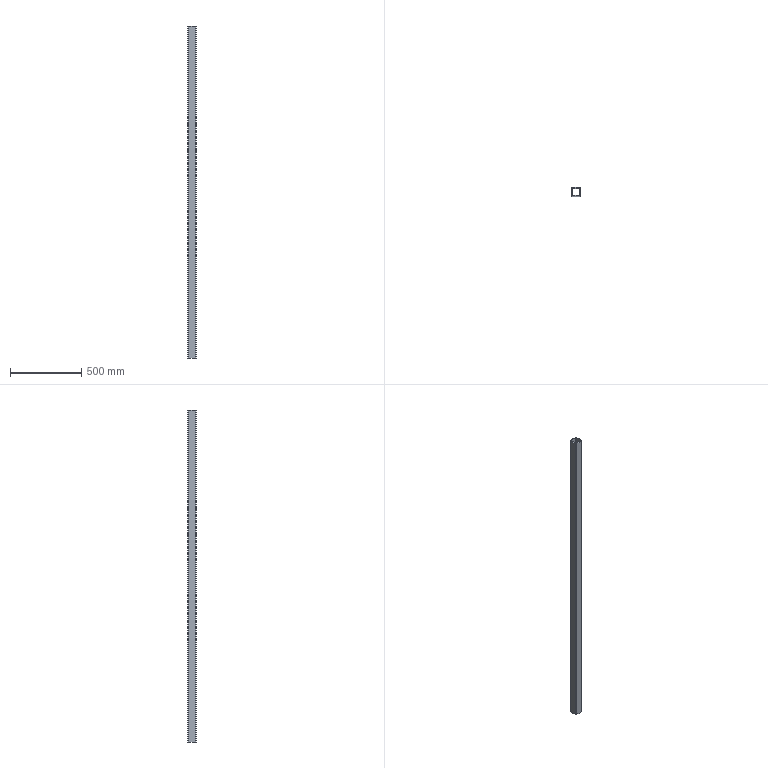Part | SolidWorks | features Fillet 2, Extrusion 1 | 1 solid | 18 faces | box 60 x 60 x 2330 mm | volume 2033678 mm3 | plane 10 | cylinder 8 | commonest cylinder face diameters 6 x4 12 x4
STEP:
#1=CARTESIAN_POINT('',(-24.,-30.,1165.));
#2=VERTEX_POINT('',#1);
#3=CARTESIAN_POINT('',(24.,-30.,1165.));
#4=VERTEX_POINT('',#3);
#5=CARTESIAN_POINT('',(-30.,-30.,1165.));
#6=DIRECTION('',(1.,0.,0.));
#7=VECTOR('',#6,1000.);
#8=LINE('',#5,#7);
#9=EDGE_CURVE('',#2,#4,#8,.T.);
#10=ORIENTED_EDGE('',*,*,#9,.T.);
#11=CARTESIAN_POINT('',(30.,-24.,1165.));
#12=VERTEX_POINT('',#11);
#13=CARTESIAN_POINT('',(24.,-24.,1165.));
#14=DIRECTION('',(0.,0.,1.));
#15=DIRECTION('',(-1.,0.,0.));
#16=AXIS2_PLACEMENT_3D('',#13,#14,#15);
#17=CIRCLE('',#16,6.);
#18=EDGE_CURVE('',#4,#12,#17,.T.);
#19=ORIENTED_EDGE('',*,*,#18,.T.);
#20=CARTESIAN_POINT('',(30.,24.,1165.));
#21=VERTEX_POINT('',#20);
#22=CARTESIAN_POINT('',(30.,-30.,1165.));
#23=DIRECTION('',(0.,1.,0.));
#24=VECTOR('',#23,1000.);
#25=LINE('',#22,#24);
#26=EDGE_CURVE('',#12,#21,#25,.T.);
#27=ORIENTED_EDGE('',*,*,#26,.T.);
#28=CARTESIAN_POINT('',(24.,30.,1165.));
#29=VERTEX_POINT('',#28);
#30=CARTESIAN_POINT('',(24.,24.,1165.));
#31=DIRECTION('',(0.,0.,1.));
#32=DIRECTION('',(-1.,0.,0.));
#33=AXIS2_PLACEMENT_3D('',#30,#31,#32);
#34=CIRCLE('',#33,6.);
#35=EDGE_CURVE('',#21,#29,#34,.T.);
#36=ORIENTED_EDGE('',*,*,#35,.T.);
#37=CARTESIAN_POINT('',(-24.,30.,1165.));
#38=VERTEX_POINT('',#37);
#39=CARTESIAN_POINT('',(-30.,30.,1165.));
#40=DIRECTION('',(-1.,0.,0.));
#41=VECTOR('',#40,1000.);
#42=LINE('',#39,#41);
#43=EDGE_CURVE('',#29,#38,#42,.T.);
#44=ORIENTED_EDGE('',*,*,#43,.T.);
#45=CARTESIAN_POINT('',(-30.,24.,1165.));
#46=VERTEX_POINT('',#45);
#47=CARTESIAN_POINT('',(-24.,24.,1165.));
#48=DIRECTION('',(0.,0.,1.));
#49=DIRECTION('',(-1.,0.,0.));
#50=AXIS2_PLACEMENT_3D('',#47,#48,#49);
#51=CIRCLE('',#50,6.);
#52=EDGE_CURVE('',#38,#46,#51,.T.);
#53=ORIENTED_EDGE('',*,*,#52,.T.);
#54=CARTESIAN_POINT('',(-30.,-24.,1165.));
#55=VERTEX_POINT('',#54);
#56=CARTESIAN_POINT('',(-30.,-30.,1165.));
#57=DIRECTION('',(0.,-1.,0.));
#58=VECTOR('',#57,1000.);
#59=LINE('',#56,#58);
#60=EDGE_CURVE('',#46,#55,#59,.T.);
#61=ORIENTED_EDGE('',*,*,#60,.T.);
#62=CARTESIAN_POINT('',(-24.,-24.,1165.));
#63=DIRECTION('',(0.,0.,1.));
#64=DIRECTION('',(-1.,0.,0.));
#65=AXIS2_PLACEMENT_3D('',#62,#63,#64);
#66=CIRCLE('',#65,6.);
#67=EDGE_CURVE('',#55,#2,#66,.T.);
#68=ORIENTED_EDGE('',*,*,#67,.T.);
#69=EDGE_LOOP('',(#10,#19,#27,#36,#44,#53,#61,#68));
#70=FACE_OUTER_BOUND('',#69,.T.);
#71=CARTESIAN_POINT('',(26.,-23.,1165.));
#72=VERTEX_POINT('',#71);
#73=CARTESIAN_POINT('',(26.,23.,1165.));
#74=VERTEX_POINT('',#73);
#75=CARTESIAN_POINT('',(26.,-26.,1165.));
#76=DIRECTION('',(0.,1.,0.));
#77=VECTOR('',#76,1000.);
#78=LINE('',#75,#77);
#79=EDGE_CURVE('',#72,#74,#78,.T.);
#80=ORIENTED_EDGE('',*,*,#79,.F.);
#81=CARTESIAN_POINT('',(23.,-26.,1165.));
#82=VERTEX_POINT('',#81);
#83=CARTESIAN_POINT('',(23.,-23.,1165.));
#84=DIRECTION('',(0.,0.,-1.));
#85=DIRECTION('',(-1.,0.,0.));
#86=AXIS2_PLACEMENT_3D('',#83,#84,#85);
#87=CIRCLE('',#86,3.);
#88=EDGE_CURVE('',#72,#82,#87,.T.);
#89=ORIENTED_EDGE('',*,*,#88,.T.);
#90=CARTESIAN_POINT('',(-23.,-26.,1165.));
#91=VERTEX_POINT('',#90);
#92=CARTESIAN_POINT('',(-26.,-26.,1165.));
#93=DIRECTION('',(1.,0.,0.));
#94=VECTOR('',#93,1000.);
#95=LINE('',#92,#94);
#96=EDGE_CURVE('',#91,#82,#95,.T.);
#97=ORIENTED_EDGE('',*,*,#96,.F.);
#98=CARTESIAN_POINT('',(-26.,-23.,1165.));
#99=VERTEX_POINT('',#98);
#100=CARTESIAN_POINT('',(-23.,-23.,1165.));
#101=DIRECTION('',(0.,0.,-1.));
#102=DIRECTION('',(-1.,0.,0.));
#103=AXIS2_PLACEMENT_3D('',#100,#101,#102);
#104=CIRCLE('',#103,3.);
#105=EDGE_CURVE('',#91,#99,#104,.T.);
#106=ORIENTED_EDGE('',*,*,#105,.T.);
#107=CARTESIAN_POINT('',(-26.,23.,1165.));
#108=VERTEX_POINT('',#107);
#109=CARTESIAN_POINT('',(-26.,-26.,1165.));
#110=DIRECTION('',(0.,-1.,0.));
#111=VECTOR('',#110,1000.);
#112=LINE('',#109,#111);
#113=EDGE_CURVE('',#108,#99,#112,.T.);
#114=ORIENTED_EDGE('',*,*,#113,.F.);
#115=CARTESIAN_POINT('',(-23.,26.,1165.));
#116=VERTEX_POINT('',#115);
#117=CARTESIAN_POINT('',(-23.,23.,1165.));
#118=DIRECTION('',(0.,0.,-1.));
#119=DIRECTION('',(-1.,0.,0.));
#120=AXIS2_PLACEMENT_3D('',#117,#118,#119);
#121=CIRCLE('',#120,3.);
#122=EDGE_CURVE('',#108,#116,#121,.T.);
#123=ORIENTED_EDGE('',*,*,#122,.T.);
#124=CARTESIAN_POINT('',(23.,26.,1165.));
#125=VERTEX_POINT('',#124);
#126=CARTESIAN_POINT('',(-26.,26.,1165.));
#127=DIRECTION('',(-1.,0.,0.));
#128=VECTOR('',#127,1000.);
#129=LINE('',#126,#128);
#130=EDGE_CURVE('',#125,#116,#129,.T.);
#131=ORIENTED_EDGE('',*,*,#130,.F.);
#132=CARTESIAN_POINT('',(23.,23.,1165.));
#133=DIRECTION('',(0.,0.,-1.));
#134=DIRECTION('',(-1.,0.,0.));
#135=AXIS2_PLACEMENT_3D('',#132,#133,#134);
#136=CIRCLE('',#135,3.);
#137=EDGE_CURVE('',#125,#74,#136,.T.);
#138=ORIENTED_EDGE('',*,*,#137,.T.);
#139=EDGE_LOOP('',(#80,#89,#97,#106,#114,#123,#131,#138));
#140=FACE_BOUND('',#139,.T.);
#141=CARTESIAN_POINT('',(0.,0.,1165.));
#142=DIRECTION('',(0.,0.,-1.));
#143=DIRECTION('',(-1.,0.,0.));
#144=AXIS2_PLACEMENT_3D('',#141,#142,#143);
#145=PLANE('',#144);
#146=ADVANCED_FACE('',(#70,#140),#145,.F.);
#147=CARTESIAN_POINT('',(30.,-24.,-1165.));
#148=VERTEX_POINT('',#147);
#149=CARTESIAN_POINT('',(30.,24.,-1165.));
#150=VERTEX_POINT('',#149);
#151=CARTESIAN_POINT('',(30.,-30.,-1165.));
#152=DIRECTION('',(0.,1.,0.));
#153=VECTOR('',#152,1000.);
#154=LINE('',#151,#153);
#155=EDGE_CURVE('',#148,#150,#154,.T.);
#156=ORIENTED_EDGE('',*,*,#155,.F.);
#157=CARTESIAN_POINT('',(24.,-30.,-1165.));
#158=VERTEX_POINT('',#157);
#159=CARTESIAN_POINT('',(24.,-24.,-1165.));
#160=DIRECTION('',(0.,0.,-1.));
#161=DIRECTION('',(-1.,0.,0.));
#162=AXIS2_PLACEMENT_3D('',#159,#160,#161);
#163=CIRCLE('',#162,6.);
#164=EDGE_CURVE('',#148,#158,#163,.T.);
#165=ORIENTED_EDGE('',*,*,#164,.T.);
#166=CARTESIAN_POINT('',(-24.,-30.,-1165.));
#167=VERTEX_POINT('',#166);
#168=CARTESIAN_POINT('',(-30.,-30.,-1165.));
#169=DIRECTION('',(1.,0.,0.));
#170=VECTOR('',#169,1000.);
#171=LINE('',#168,#170);
#172=EDGE_CURVE('',#167,#158,#171,.T.);
#173=ORIENTED_EDGE('',*,*,#172,.F.);
#174=CARTESIAN_POINT('',(-30.,-24.,-1165.));
#175=VERTEX_POINT('',#174);
#176=CARTESIAN_POINT('',(-24.,-24.,-1165.));
#177=DIRECTION('',(0.,0.,-1.));
#178=DIRECTION('',(-1.,0.,0.));
#179=AXIS2_PLACEMENT_3D('',#176,#177,#178);
#180=CIRCLE('',#179,6.);
#181=EDGE_CURVE('',#167,#175,#180,.T.);
#182=ORIENTED_EDGE('',*,*,#181,.T.);
#183=CARTESIAN_POINT('',(-30.,24.,-1165.));
#184=VERTEX_POINT('',#183);
#185=CARTESIAN_POINT('',(-30.,-30.,-1165.));
#186=DIRECTION('',(0.,-1.,0.));
#187=VECTOR('',#186,1000.);
#188=LINE('',#185,#187);
#189=EDGE_CURVE('',#184,#175,#188,.T.);
#190=ORIENTED_EDGE('',*,*,#189,.F.);
#191=CARTESIAN_POINT('',(-24.,30.,-1165.));
#192=VERTEX_POINT('',#191);
#193=CARTESIAN_POINT('',(-24.,24.,-1165.));
#194=DIRECTION('',(0.,0.,-1.));
#195=DIRECTION('',(-1.,0.,0.));
#196=AXIS2_PLACEMENT_3D('',#193,#194,#195);
#197=CIRCLE('',#196,6.);
#198=EDGE_CURVE('',#184,#192,#197,.T.);
#199=ORIENTED_EDGE('',*,*,#198,.T.);
#200=CARTESIAN_POINT('',(24.,30.,-1165.));
#201=VERTEX_POINT('',#200);
#202=CARTESIAN_POINT('',(-30.,30.,-1165.));
#203=DIRECTION('',(-1.,0.,0.));
#204=VECTOR('',#203,1000.);
#205=LINE('',#202,#204);
#206=EDGE_CURVE('',#201,#192,#205,.T.);
#207=ORIENTED_EDGE('',*,*,#206,.F.);
#208=CARTESIAN_POINT('',(24.,24.,-1165.));
#209=DIRECTION('',(0.,0.,-1.));
#210=DIRECTION('',(-1.,0.,0.));
#211=AXIS2_PLACEMENT_3D('',#208,#209,#210);
#212=CIRCLE('',#211,6.);
#213=EDGE_CURVE('',#201,#150,#212,.T.);
#214=ORIENTED_EDGE('',*,*,#213,.T.);
#215=EDGE_LOOP('',(#156,#165,#173,#182,#190,#199,#207,#214));
#216=FACE_OUTER_BOUND('',#215,.T.);
#217=CARTESIAN_POINT('',(-26.,23.,-1165.));
#218=VERTEX_POINT('',#217);
#219=CARTESIAN_POINT('',(-26.,-23.,-1165.));
#220=VERTEX_POINT('',#219);
#221=CARTESIAN_POINT('',(-26.,-26.,-1165.));
#222=DIRECTION('',(0.,-1.,0.));
#223=VECTOR('',#222,1000.);
#224=LINE('',#221,#223);
#225=EDGE_CURVE('',#218,#220,#224,.T.);
#226=ORIENTED_EDGE('',*,*,#225,.T.);
#227=CARTESIAN_POINT('',(-23.,-26.,-1165.));
#228=VERTEX_POINT('',#227);
#229=CARTESIAN_POINT('',(-23.,-23.,-1165.));
#230=DIRECTION('',(0.,0.,1.));
#231=DIRECTION('',(-1.,0.,0.));
#232=AXIS2_PLACEMENT_3D('',#229,#230,#231);
#233=CIRCLE('',#232,3.);
#234=EDGE_CURVE('',#220,#228,#233,.T.);
#235=ORIENTED_EDGE('',*,*,#234,.T.);
#236=CARTESIAN_POINT('',(23.,-26.,-1165.));
#237=VERTEX_POINT('',#236);
#238=CARTESIAN_POINT('',(-26.,-26.,-1165.));
#239=DIRECTION('',(1.,0.,0.));
#240=VECTOR('',#239,1000.);
#241=LINE('',#238,#240);
#242=EDGE_CURVE('',#228,#237,#241,.T.);
#243=ORIENTED_EDGE('',*,*,#242,.T.);
#244=CARTESIAN_POINT('',(26.,-23.,-1165.));
#245=VERTEX_POINT('',#244);
#246=CARTESIAN_POINT('',(23.,-23.,-1165.));
#247=DIRECTION('',(0.,0.,1.));
#248=DIRECTION('',(-1.,0.,0.));
#249=AXIS2_PLACEMENT_3D('',#246,#247,#248);
#250=CIRCLE('',#249,3.);
#251=EDGE_CURVE('',#237,#245,#250,.T.);
#252=ORIENTED_EDGE('',*,*,#251,.T.);
#253=CARTESIAN_POINT('',(26.,23.,-1165.));
#254=VERTEX_POINT('',#253);
#255=CARTESIAN_POINT('',(26.,-26.,-1165.));
#256=DIRECTION('',(0.,1.,0.));
#257=VECTOR('',#256,1000.);
#258=LINE('',#255,#257);
#259=EDGE_CURVE('',#245,#254,#258,.T.);
#260=ORIENTED_EDGE('',*,*,#259,.T.);
#261=CARTESIAN_POINT('',(23.,26.,-1165.));
#262=VERTEX_POINT('',#261);
#263=CARTESIAN_POINT('',(23.,23.,-1165.));
#264=DIRECTION('',(0.,0.,1.));
#265=DIRECTION('',(-1.,0.,0.));
#266=AXIS2_PLACEMENT_3D('',#263,#264,#265);
#267=CIRCLE('',#266,3.);
#268=EDGE_CURVE('',#254,#262,#267,.T.);
#269=ORIENTED_EDGE('',*,*,#268,.T.);
#270=CARTESIAN_POINT('',(-23.,26.,-1165.));
#271=VERTEX_POINT('',#270);
#272=CARTESIAN_POINT('',(-26.,26.,-1165.));
#273=DIRECTION('',(-1.,0.,0.));
#274=VECTOR('',#273,1000.);
#275=LINE('',#272,#274);
#276=EDGE_CURVE('',#262,#271,#275,.T.);
#277=ORIENTED_EDGE('',*,*,#276,.T.);
#278=CARTESIAN_POINT('',(-23.,23.,-1165.));
#279=DIRECTION('',(0.,0.,1.));
#280=DIRECTION('',(-1.,0.,0.));
#281=AXIS2_PLACEMENT_3D('',#278,#279,#280);
#282=CIRCLE('',#281,3.);
#283=EDGE_CURVE('',#271,#218,#282,.T.);
#284=ORIENTED_EDGE('',*,*,#283,.T.);
#285=EDGE_LOOP('',(#226,#235,#243,#252,#260,#269,#277,#284));
#286=FACE_BOUND('',#285,.T.);
#287=CARTESIAN_POINT('',(0.,0.,-1165.));
#288=DIRECTION('',(0.,0.,-1.));
#289=DIRECTION('',(-1.,0.,0.));
#290=AXIS2_PLACEMENT_3D('',#287,#288,#289);
#291=PLANE('',#290);
#292=ADVANCED_FACE('',(#216,#286),#291,.T.);
#293=ORIENTED_EDGE('',*,*,#26,.F.);
#294=CARTESIAN_POINT('',(30.,-24.,1165.));
#295=DIRECTION('',(0.,0.,-1.));
#296=VECTOR('',#295,1000.);
#297=LINE('',#294,#296);
#298=EDGE_CURVE('',#12,#148,#297,.T.);
#299=ORIENTED_EDGE('',*,*,#298,.T.);
#300=ORIENTED_EDGE('',*,*,#155,.T.);
#301=CARTESIAN_POINT('',(30.,24.,1165.));
#302=DIRECTION('',(0.,0.,1.));
#303=VECTOR('',#302,1000.);
#304=LINE('',#301,#303);
#305=EDGE_CURVE('',#150,#21,#304,.T.);
#306=ORIENTED_EDGE('',*,*,#305,.T.);
#307=EDGE_LOOP('',(#293,#299,#300,#306));
#308=FACE_OUTER_BOUND('',#307,.T.);
#309=CARTESIAN_POINT('',(30.,-30.,1165.));
#310=DIRECTION('',(-1.,0.,0.));
#311=DIRECTION('',(0.,0.,1.));
#312=AXIS2_PLACEMENT_3D('',#309,#310,#311);
#313=PLANE('',#312);
#314=ADVANCED_FACE('',(#308),#313,.F.);
#315=ORIENTED_EDGE('',*,*,#43,.F.);
#316=CARTESIAN_POINT('',(24.,30.,1165.));
#317=DIRECTION('',(0.,0.,-1.));
#318=VECTOR('',#317,1000.);
#319=LINE('',#316,#318);
#320=EDGE_CURVE('',#29,#201,#319,.T.);
#321=ORIENTED_EDGE('',*,*,#320,.T.);
#322=ORIENTED_EDGE('',*,*,#206,.T.);
#323=CARTESIAN_POINT('',(-24.,30.,1165.));
#324=DIRECTION('',(0.,0.,1.));
#325=VECTOR('',#324,1000.);
#326=LINE('',#323,#325);
#327=EDGE_CURVE('',#192,#38,#326,.T.);
#328=ORIENTED_EDGE('',*,*,#327,.T.);
#329=EDGE_LOOP('',(#315,#321,#322,#328));
#330=FACE_OUTER_BOUND('',#329,.T.);
#331=CARTESIAN_POINT('',(-30.,30.,1165.));
#332=DIRECTION('',(0.,-1.,0.));
#333=DIRECTION('',(0.,0.,-1.));
#334=AXIS2_PLACEMENT_3D('',#331,#332,#333);
#335=PLANE('',#334);
#336=ADVANCED_FACE('',(#330),#335,.F.);
#337=ORIENTED_EDGE('',*,*,#189,.T.);
#338=CARTESIAN_POINT('',(-30.,-24.,1165.));
#339=DIRECTION('',(0.,0.,1.));
#340=VECTOR('',#339,1000.);
#341=LINE('',#338,#340);
#342=EDGE_CURVE('',#175,#55,#341,.T.);
#343=ORIENTED_EDGE('',*,*,#342,.T.);
#344=ORIENTED_EDGE('',*,*,#60,.F.);
#345=CARTESIAN_POINT('',(-30.,24.,1165.));
#346=DIRECTION('',(0.,0.,-1.));
#347=VECTOR('',#346,1000.);
#348=LINE('',#345,#347);
#349=EDGE_CURVE('',#46,#184,#348,.T.);
#350=ORIENTED_EDGE('',*,*,#349,.T.);
#351=EDGE_LOOP('',(#337,#343,#344,#350));
#352=FACE_OUTER_BOUND('',#351,.T.);
#353=CARTESIAN_POINT('',(-30.,-30.,1165.));
#354=DIRECTION('',(1.,0.,0.));
#355=DIRECTION('',(0.,0.,-1.));
#356=AXIS2_PLACEMENT_3D('',#353,#354,#355);
#357=PLANE('',#356);
#358=ADVANCED_FACE('',(#352),#357,.F.);
#359=ORIENTED_EDGE('',*,*,#172,.T.);
#360=CARTESIAN_POINT('',(24.,-30.,1165.));
#361=DIRECTION('',(0.,0.,1.));
#362=VECTOR('',#361,1000.);
#363=LINE('',#360,#362);
#364=EDGE_CURVE('',#158,#4,#363,.T.);
#365=ORIENTED_EDGE('',*,*,#364,.T.);
#366=ORIENTED_EDGE('',*,*,#9,.F.);
#367=CARTESIAN_POINT('',(-24.,-30.,1165.));
#368=DIRECTION('',(0.,0.,-1.));
#369=VECTOR('',#368,1000.);
#370=LINE('',#367,#369);
#371=EDGE_CURVE('',#2,#167,#370,.T.);
#372=ORIENTED_EDGE('',*,*,#371,.T.);
#373=EDGE_LOOP('',(#359,#365,#366,#372));
#374=FACE_OUTER_BOUND('',#373,.T.);
#375=CARTESIAN_POINT('',(-30.,-30.,1165.));
#376=DIRECTION('',(0.,1.,0.));
#377=DIRECTION('',(0.,0.,1.));
#378=AXIS2_PLACEMENT_3D('',#375,#376,#377);
#379=PLANE('',#378);
#380=ADVANCED_FACE('',(#374),#379,.F.);
#381=ORIENTED_EDGE('',*,*,#259,.F.);
#382=CARTESIAN_POINT('',(26.,-23.,1165.));
#383=DIRECTION('',(0.,0.,1.));
#384=VECTOR('',#383,1000.);
#385=LINE('',#382,#384);
#386=EDGE_CURVE('',#245,#72,#385,.T.);
#387=ORIENTED_EDGE('',*,*,#386,.T.);
#388=ORIENTED_EDGE('',*,*,#79,.T.);
#389=CARTESIAN_POINT('',(26.,23.,-1165.));
#390=DIRECTION('',(0.,0.,-1.));
#391=VECTOR('',#390,1000.);
#392=LINE('',#389,#391);
#393=EDGE_CURVE('',#74,#254,#392,.T.);
#394=ORIENTED_EDGE('',*,*,#393,.T.);
#395=EDGE_LOOP('',(#381,#387,#388,#394));
#396=FACE_OUTER_BOUND('',#395,.T.);
#397=CARTESIAN_POINT('',(26.,-26.,1165.));
#398=DIRECTION('',(-1.,0.,0.));
#399=DIRECTION('',(0.,0.,1.));
#400=AXIS2_PLACEMENT_3D('',#397,#398,#399);
#401=PLANE('',#400);
#402=ADVANCED_FACE('',(#396),#401,.T.);
#403=ORIENTED_EDGE('',*,*,#276,.F.);
#404=CARTESIAN_POINT('',(23.,26.,1165.));
#405=DIRECTION('',(0.,0.,1.));
#406=VECTOR('',#405,1000.);
#407=LINE('',#404,#406);
#408=EDGE_CURVE('',#262,#125,#407,.T.);
#409=ORIENTED_EDGE('',*,*,#408,.T.);
#410=ORIENTED_EDGE('',*,*,#130,.T.);
#411=CARTESIAN_POINT('',(-23.,26.,-1165.));
#412=DIRECTION('',(0.,0.,-1.));
#413=VECTOR('',#412,1000.);
#414=LINE('',#411,#413);
#415=EDGE_CURVE('',#116,#271,#414,.T.);
#416=ORIENTED_EDGE('',*,*,#415,.T.);
#417=EDGE_LOOP('',(#403,#409,#410,#416));
#418=FACE_OUTER_BOUND('',#417,.T.);
#419=CARTESIAN_POINT('',(-26.,26.,1165.));
#420=DIRECTION('',(0.,-1.,0.));
#421=DIRECTION('',(0.,0.,-1.));
#422=AXIS2_PLACEMENT_3D('',#419,#420,#421);
#423=PLANE('',#422);
#424=ADVANCED_FACE('',(#418),#423,.T.);
#425=ORIENTED_EDGE('',*,*,#113,.T.);
#426=CARTESIAN_POINT('',(-26.,-23.,-1165.));
#427=DIRECTION('',(0.,0.,-1.));
#428=VECTOR('',#427,1000.);
#429=LINE('',#426,#428);
#430=EDGE_CURVE('',#99,#220,#429,.T.);
#431=ORIENTED_EDGE('',*,*,#430,.T.);
#432=ORIENTED_EDGE('',*,*,#225,.F.);
#433=CARTESIAN_POINT('',(-26.,23.,1165.));
#434=DIRECTION('',(0.,0.,1.));
#435=VECTOR('',#434,1000.);
#436=LINE('',#433,#435);
#437=EDGE_CURVE('',#218,#108,#436,.T.);
#438=ORIENTED_EDGE('',*,*,#437,.T.);
#439=EDGE_LOOP('',(#425,#431,#432,#438));
#440=FACE_OUTER_BOUND('',#439,.T.);
#441=CARTESIAN_POINT('',(-26.,-26.,1165.));
#442=DIRECTION('',(1.,0.,0.));
#443=DIRECTION('',(0.,0.,-1.));
#444=AXIS2_PLACEMENT_3D('',#441,#442,#443);
#445=PLANE('',#444);
#446=ADVANCED_FACE('',(#440),#445,.T.);
#447=ORIENTED_EDGE('',*,*,#96,.T.);
#448=CARTESIAN_POINT('',(23.,-26.,-1165.));
#449=DIRECTION('',(0.,0.,-1.));
#450=VECTOR('',#449,1000.);
#451=LINE('',#448,#450);
#452=EDGE_CURVE('',#82,#237,#451,.T.);
#453=ORIENTED_EDGE('',*,*,#452,.T.);
#454=ORIENTED_EDGE('',*,*,#242,.F.);
#455=CARTESIAN_POINT('',(-23.,-26.,1165.));
#456=DIRECTION('',(0.,0.,1.));
#457=VECTOR('',#456,1000.);
#458=LINE('',#455,#457);
#459=EDGE_CURVE('',#228,#91,#458,.T.);
#460=ORIENTED_EDGE('',*,*,#459,.T.);
#461=EDGE_LOOP('',(#447,#453,#454,#460));
#462=FACE_OUTER_BOUND('',#461,.T.);
#463=CARTESIAN_POINT('',(-26.,-26.,1165.));
#464=DIRECTION('',(0.,1.,0.));
#465=DIRECTION('',(0.,0.,1.));
#466=AXIS2_PLACEMENT_3D('',#463,#464,#465);
#467=PLANE('',#466);
#468=ADVANCED_FACE('',(#462),#467,.T.);
#469=ORIENTED_EDGE('',*,*,#18,.F.);
#470=ORIENTED_EDGE('',*,*,#364,.F.);
#471=ORIENTED_EDGE('',*,*,#164,.F.);
#472=ORIENTED_EDGE('',*,*,#298,.F.);
#473=EDGE_LOOP('',(#469,#470,#471,#472));
#474=FACE_OUTER_BOUND('',#473,.T.);
#475=CARTESIAN_POINT('',(24.,-24.,1165.));
#476=DIRECTION('',(0.,0.,-1.));
#477=DIRECTION('',(-1.,0.,0.));
#478=AXIS2_PLACEMENT_3D('',#475,#476,#477);
#479=CYLINDRICAL_SURFACE('',#478,6.);
#480=ADVANCED_FACE('',(#474),#479,.T.);
#481=ORIENTED_EDGE('',*,*,#67,.F.);
#482=ORIENTED_EDGE('',*,*,#342,.F.);
#483=ORIENTED_EDGE('',*,*,#181,.F.);
#484=ORIENTED_EDGE('',*,*,#371,.F.);
#485=EDGE_LOOP('',(#481,#482,#483,#484));
#486=FACE_OUTER_BOUND('',#485,.T.);
#487=CARTESIAN_POINT('',(-24.,-24.,1165.));
#488=DIRECTION('',(0.,0.,-1.));
#489=DIRECTION('',(-1.,0.,0.));
#490=AXIS2_PLACEMENT_3D('',#487,#488,#489);
#491=CYLINDRICAL_SURFACE('',#490,6.);
#492=ADVANCED_FACE('',(#486),#491,.T.);
#493=ORIENTED_EDGE('',*,*,#35,.F.);
#494=ORIENTED_EDGE('',*,*,#305,.F.);
#495=ORIENTED_EDGE('',*,*,#213,.F.);
#496=ORIENTED_EDGE('',*,*,#320,.F.);
#497=EDGE_LOOP('',(#493,#494,#495,#496));
#498=FACE_OUTER_BOUND('',#497,.T.);
#499=CARTESIAN_POINT('',(24.,24.,1165.));
#500=DIRECTION('',(0.,0.,-1.));
#501=DIRECTION('',(-1.,0.,0.));
#502=AXIS2_PLACEMENT_3D('',#499,#500,#501);
#503=CYLINDRICAL_SURFACE('',#502,6.);
#504=ADVANCED_FACE('',(#498),#503,.T.);
#505=ORIENTED_EDGE('',*,*,#52,.F.);
#506=ORIENTED_EDGE('',*,*,#327,.F.);
#507=ORIENTED_EDGE('',*,*,#198,.F.);
#508=ORIENTED_EDGE('',*,*,#349,.F.);
#509=EDGE_LOOP('',(#505,#506,#507,#508));
#510=FACE_OUTER_BOUND('',#509,.T.);
#511=CARTESIAN_POINT('',(-24.,24.,1165.));
#512=DIRECTION('',(0.,0.,-1.));
#513=DIRECTION('',(-1.,0.,0.));
#514=AXIS2_PLACEMENT_3D('',#511,#512,#513);
#515=CYLINDRICAL_SURFACE('',#514,6.);
#516=ADVANCED_FACE('',(#510),#515,.T.);
#517=ORIENTED_EDGE('',*,*,#88,.F.);
#518=ORIENTED_EDGE('',*,*,#386,.F.);
#519=ORIENTED_EDGE('',*,*,#251,.F.);
#520=ORIENTED_EDGE('',*,*,#452,.F.);
#521=EDGE_LOOP('',(#517,#518,#519,#520));
#522=FACE_OUTER_BOUND('',#521,.T.);
#523=CARTESIAN_POINT('',(23.,-23.,1165.));
#524=DIRECTION('',(0.,0.,1.));
#525=DIRECTION('',(1.,0.,0.));
#526=AXIS2_PLACEMENT_3D('',#523,#524,#525);
#527=CYLINDRICAL_SURFACE('',#526,3.);
#528=ADVANCED_FACE('',(#522),#527,.F.);
#529=ORIENTED_EDGE('',*,*,#105,.F.);
#530=ORIENTED_EDGE('',*,*,#459,.F.);
#531=ORIENTED_EDGE('',*,*,#234,.F.);
#532=ORIENTED_EDGE('',*,*,#430,.F.);
#533=EDGE_LOOP('',(#529,#530,#531,#532));
#534=FACE_OUTER_BOUND('',#533,.T.);
#535=CARTESIAN_POINT('',(-23.,-23.,1165.));
#536=DIRECTION('',(0.,0.,1.));
#537=DIRECTION('',(1.,0.,0.));
#538=AXIS2_PLACEMENT_3D('',#535,#536,#537);
#539=CYLINDRICAL_SURFACE('',#538,3.);
#540=ADVANCED_FACE('',(#534),#539,.F.);
#541=ORIENTED_EDGE('',*,*,#137,.F.);
#542=ORIENTED_EDGE('',*,*,#408,.F.);
#543=ORIENTED_EDGE('',*,*,#268,.F.);
#544=ORIENTED_EDGE('',*,*,#393,.F.);
#545=EDGE_LOOP('',(#541,#542,#543,#544));
#546=FACE_OUTER_BOUND('',#545,.T.);
#547=CARTESIAN_POINT('',(23.,23.,1165.));
#548=DIRECTION('',(0.,0.,1.));
#549=DIRECTION('',(1.,0.,0.));
#550=AXIS2_PLACEMENT_3D('',#547,#548,#549);
#551=CYLINDRICAL_SURFACE('',#550,3.);
#552=ADVANCED_FACE('',(#546),#551,.F.);
#553=ORIENTED_EDGE('',*,*,#122,.F.);
#554=ORIENTED_EDGE('',*,*,#437,.F.);
#555=ORIENTED_EDGE('',*,*,#283,.F.);
#556=ORIENTED_EDGE('',*,*,#415,.F.);
#557=EDGE_LOOP('',(#553,#554,#555,#556));
#558=FACE_OUTER_BOUND('',#557,.T.);
#559=CARTESIAN_POINT('',(-23.,23.,1165.));
#560=DIRECTION('',(0.,0.,1.));
#561=DIRECTION('',(1.,0.,0.));
#562=AXIS2_PLACEMENT_3D('',#559,#560,#561);
#563=CYLINDRICAL_SURFACE('',#562,3.);
#564=ADVANCED_FACE('',(#558),#563,.F.);
#565=CLOSED_SHELL('',(#146,#292,#314,#336,#358,#380,#402,#424,#446,#468,#480,#492,#504,#516,#528,#540,#552,#564));
#566=MANIFOLD_SOLID_BREP('',#565);
#567=CARTESIAN_POINT('',(0.,0.,0.));
#568=DIRECTION('',(0.,0.,1.));
#569=DIRECTION('',(1.,0.,0.));
#570=AXIS2_PLACEMENT_3D('',#567,#568,#569);
#571=(LENGTH_UNIT()NAMED_UNIT(*)SI_UNIT(.MILLI.,.METRE.));
#572=UNCERTAINTY_MEASURE_WITH_UNIT(LENGTH_MEASURE(0.00001),#571,'','');
#573=(NAMED_UNIT(*)PLANE_ANGLE_UNIT()SI_UNIT($,.RADIAN.));
#574=(NAMED_UNIT(*)SI_UNIT($,.STERADIAN.)SOLID_ANGLE_UNIT());
#575=(GEOMETRIC_REPRESENTATION_CONTEXT(3)GLOBAL_UNCERTAINTY_ASSIGNED_CONTEXT((#572))GLOBAL_UNIT_ASSIGNED_CONTEXT((#571,#573,#574))REPRESENTATION_CONTEXT('',''));
#576=ADVANCED_BREP_SHAPE_REPRESENTATION('',(#566,#570),#575);